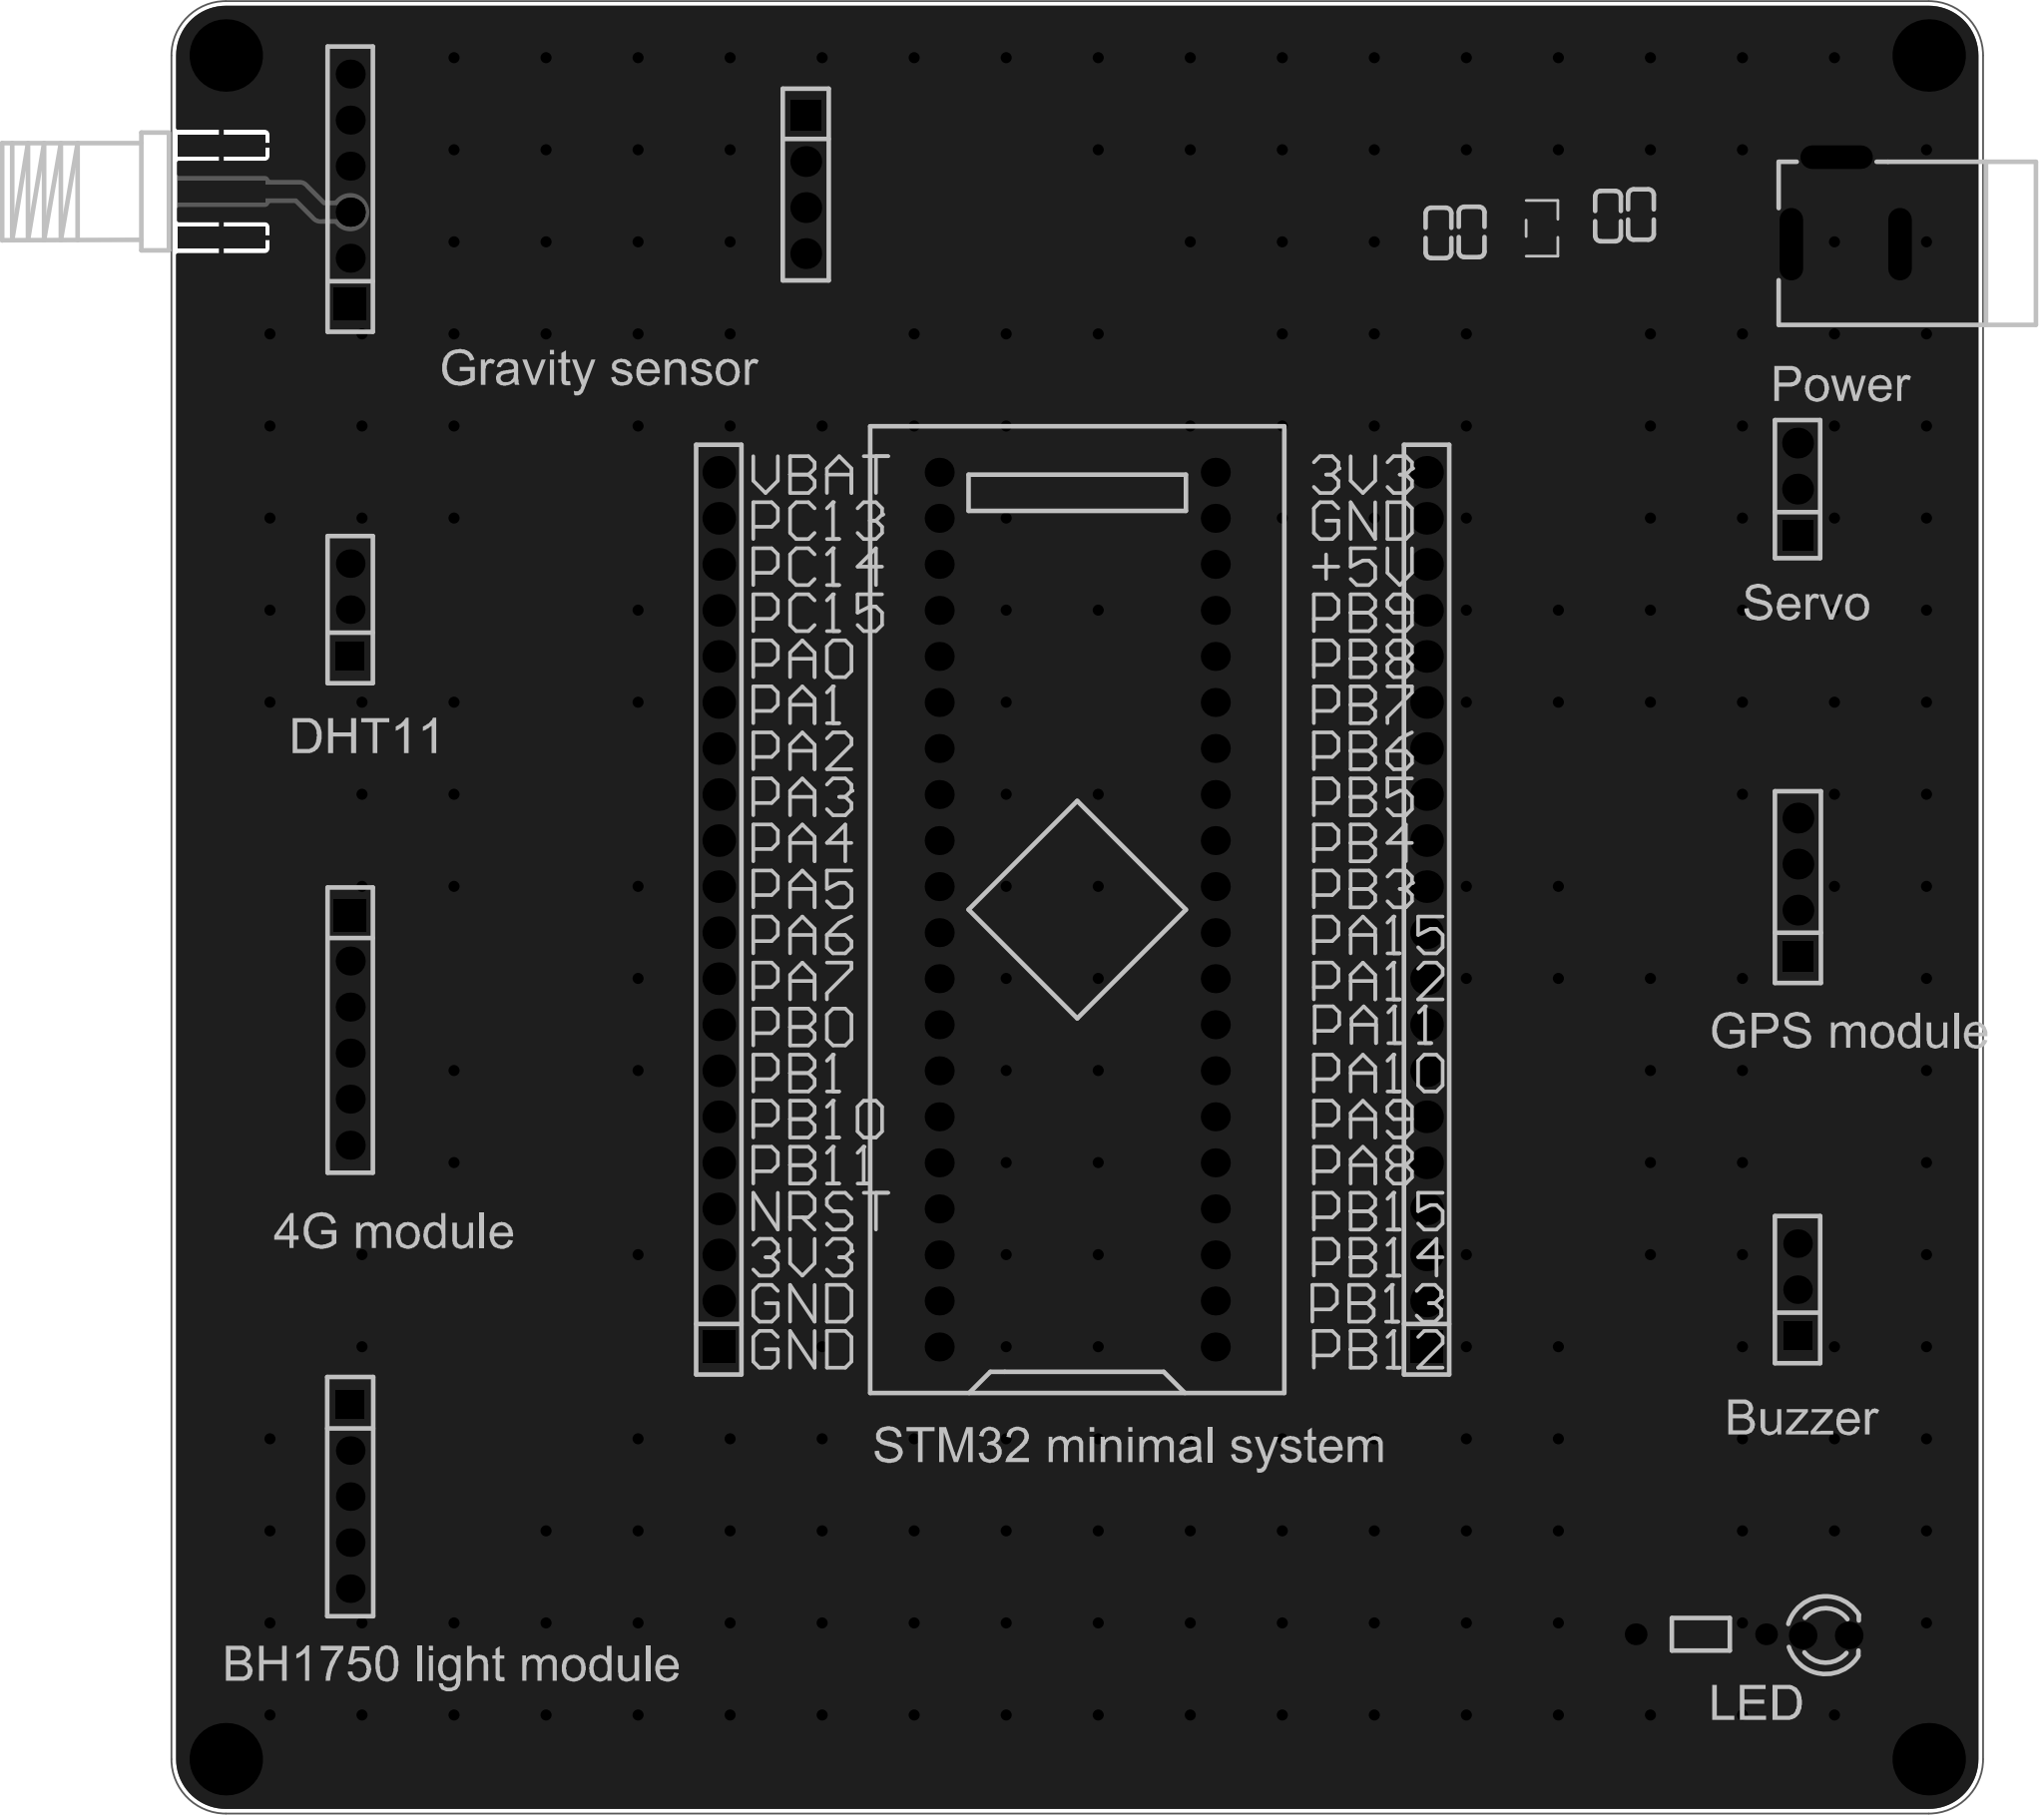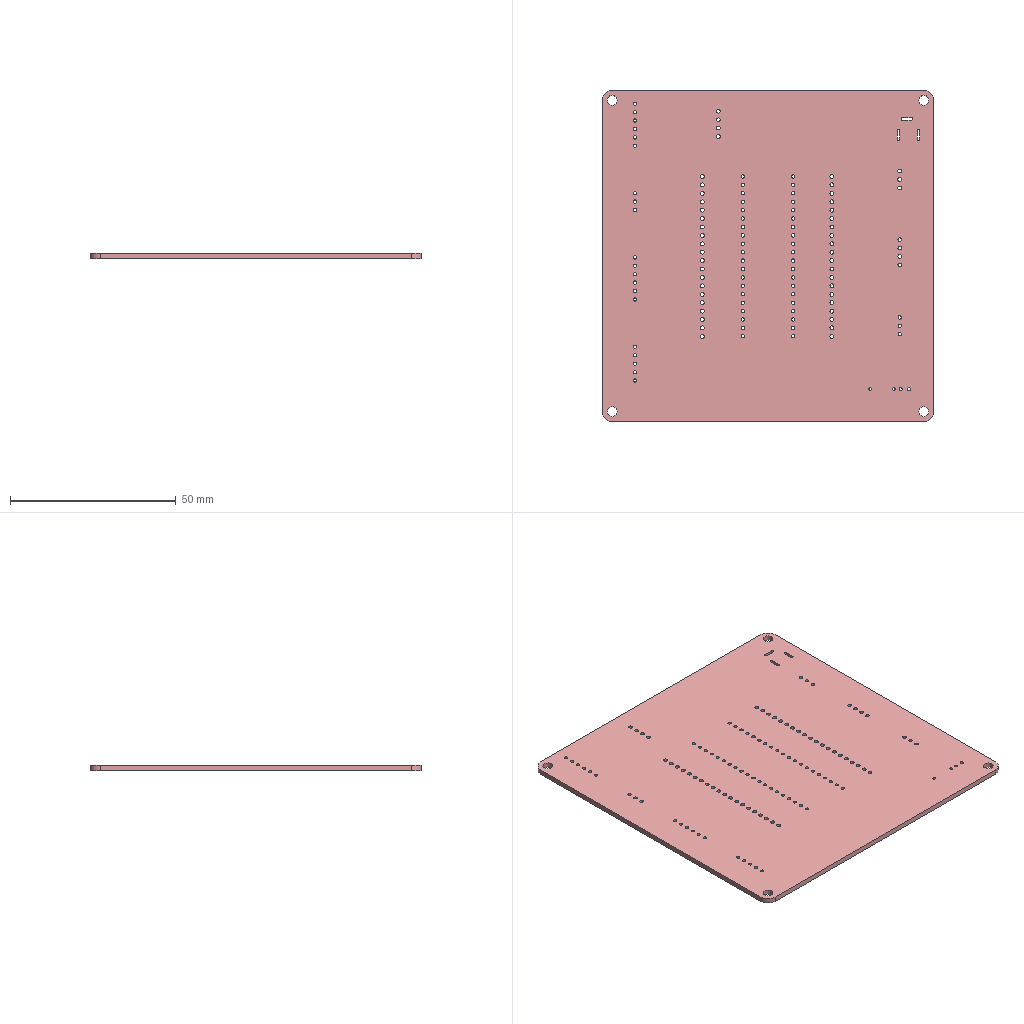Circuit board layout | Altium Designer | box 100 x 100 x 1.6 mm
Layer stack:
# Altium Designer layer stack of  (unit mm; dielectric type: 0 none, 1 core, 2 prepreg, 3 surface material)
index,name,kind,layer,copper_thickness_mm,dielectric_type,dielectric_thickness_mm,dielectric_material,dielectric_constant
0,Top Paste Mask Layer,other,,,,,,
1,Top Silkscreen Layer,other,,,,,,
2,Top Solder Mask Layer,dielectric,,,3,0.01,,3.3
3,Top Layer,copper,Top Layer,0.035,,,,
4,Dielectric1,dielectric,,,3,1.51,FR4,4.5
5,Bottom Layer,copper,Bottom Layer,0.035,,,,
6,Bottom Solder Mask Layer,dielectric,,,3,0.01,,3.3
7,Bottom Silkscreen Layer,other,,,,,,
8,Bottom Paste Mask Layer,other,,,,,,
# drill layer pairs: low layer,high layer
drill_pair,Top Layer,Bottom Layer
Part placement:
Designator,Comment,Layer,Footprint,Center-X(mm),Center-Y(mm),Rotation
U1,STM32F103C8T6-Card,TopLayer,CONN-TH_L53.3-W22.9_STM32F103C8T6-CARD,135.664,128.778,90
H1,,TopLayer,HDR-TH_20P-P2.54-V-F,154.947,128.778,90
H2,,TopLayer,HDR-TH_20P-P2.54-V-F,115.876,128.778,90
C1,10uF,TopLayer,C0603,166.779,167.132,270
C2,100nF,TopLayer,C0603,164.962,167.043,270
C3,10uF,TopLayer,C0603,157.434,166.169,270
C4,100nF,TopLayer,C0603,155.603,166.116,270
DC1,,TopLayer,DC-2.0,178.082,167.894,0
H7,,TopLayer,HDR-TH_3P-P2.54-V-F,175.424,107.811,90
U2,HT7333,TopLayer,SOT-23-3_L2.9-W1.6-P1.90-LS2.8-BR,161.318,166.37,180
H3,,TopLayer,HDR-TH_5P-P2.54-V-F,95.532,96.393,270
H8,,TopLayer,HDR-TH_3P-P2.54-V-F,95.532,145.33,90
H9,,TopLayer,HDR-TH_4P-P2.54-V-F,120.678,168.783,270
H10,,TopLayer,HDR-TH_6P-P2.54-V-F,95.532,168.529,90
H11,,TopLayer,HDR-TH_6P-P2.54-V-F,95.532,122.132,270
H12,,TopLayer,HDR-TH_3P-P2.54-V-M,175.424,151.98,90
H13,,TopLayer,HDR-TH_4P-P2.54-V-F,175.444,130.02,90
LED1,,TopLayer,LED_TH-3mm,176.976,88.734,0
R1,220,TopLayer,Res_1/8W,170.086,88.796,0
RF1,-,TopLayer,SMA-SMD_BWSMA-KE-P001,88.42,168.402,180
Pad and via stacks:
# Altium Designer via and pad stacks of  (unit mm). Each distinct definition once, with the count of objects using it.
# via: kind,start_layer,end_layer,hole_mm,diameter_mm,mode(0 simple;1 top-mid-bottom;2 full stack),diameter_per_layer,count,example_net
# pad: kind,layer,hole_mm,hole_type(0 round;1 square;2 slot),plating,top_size,top_shape(1 round;2 rect;3 octagon;9 rounded rect),mid_size,bottom_size,mode,footprint,size_per_layer,count,example
pad,Multi-Layer,3,0,plated,4x4,1,4x4,4x4,0,,,4,1
pad,Multi-Layer,1,0,plated,1.6x1.6,1,1.6x1.6,1.6x1.6,0,CONN-TH_L53.3-W22.9_STM32F103C8T6-CARD,,40,U1.1
pad,Multi-Layer,1.2,0,plated,1.8x1.8,2,1.8x1.8,1.8x1.8,0,HDR-TH_20P-P2.54-V-F,,2,H1.1
pad,Multi-Layer,1.2,0,plated,1.8x1.8,1,1.8x1.8,1.8x1.8,0,HDR-TH_20P-P2.54-V-F,,38,H1.2
pad,Multi-Layer,0.8001,2,plated,4x1.3,1,4x1.3,4x1.3,0,DC-2.0,,3,DC1.2
pad,Multi-Layer,1.02,0,plated,1.575x1.575,1,1.575x1.575,1.575x1.575,0,HDR-TH_3P-P2.54-V-F,,4,H7.3
pad,Multi-Layer,1.02,0,plated,1.575x1.575,2,1.575x1.575,1.575x1.575,0,HDR-TH_3P-P2.54-V-F,,2,H7.1
pad,Multi-Layer,1.02,0,plated,1.575x1.575,1,1.575x1.575,1.575x1.575,0,HDR-TH_5P-P2.54-V-F,,4,H3.5
pad,Multi-Layer,1.02,0,plated,1.575x1.575,2,1.575x1.575,1.575x1.575,0,HDR-TH_5P-P2.54-V-F,,1,H3.1
pad,Multi-Layer,1.1,0,plated,1.7x1.7,2,1.7x1.7,1.7x1.7,0,HDR-TH_4P-P2.54-V-F,,2,H9.1
pad,Multi-Layer,1.1,0,plated,1.7x1.7,1,1.7x1.7,1.7x1.7,0,HDR-TH_4P-P2.54-V-F,,6,H9.2
pad,Multi-Layer,1.02,0,plated,1.6x1.6,1,1.6x1.6,1.6x1.6,0,HDR-TH_6P-P2.54-V-F,,10,H10.6
pad,Multi-Layer,1.02,0,plated,1.8x1.8,2,1.8x1.8,1.8x1.8,0,HDR-TH_6P-P2.54-V-F,,2,H10.1
pad,Multi-Layer,1.1,0,plated,1.7x1.7,2,1.7x1.7,1.7x1.7,0,HDR-TH_3P-P2.54-V-M,,1,H12.1
pad,Multi-Layer,1.1,0,plated,1.7x1.7,1,1.7x1.7,1.7x1.7,0,HDR-TH_3P-P2.54-V-M,,2,H12.2
pad,Multi-Layer,0.9144,0,plated,1.524x1.524,1,1.524x1.524,1.524x1.524,0,LED_TH-3mm,,2,LED1.1
pad,Multi-Layer,0.8001,0,plated,1.199x1.199,1,1.199x1.199,1.199x1.199,0,Res_1/8W,,2,R1.1
pad,Top Layer,0,0,plated,0.8x0.9,2,0.8x0.9,0.8x0.9,0,C0603,,8,C1.2
pad,Top Layer,0,0,plated,1.07x0.6,2,1.07x0.6,1.07x0.6,0,SOT-23-3_L2.9-W1.6-P1.90-LS2.8-BR,,3,U2.1
pad,Top Layer,0,0,plated,4.8x1.2,2,4.8x1.2,4.8x1.2,0,SMA-SMD_BWSMA-KE-P001,,3,RF1.1
pad,Bottom Layer,0,0,plated,4.8x1.2,2,4.8x1.2,4.8x1.2,0,SMA-SMD_BWSMA-KE-P001,,2,RF1.3
via,Top Layer,Bottom Layer,0.3048,0.61,0,,222,GND
Copper pours:
name,layer,net,type(0 solid;1 hatched;2 none)
Bottom Layer-GND,Bottom Layer,GND,0
Top Layer-GND,Top Layer,GND,0